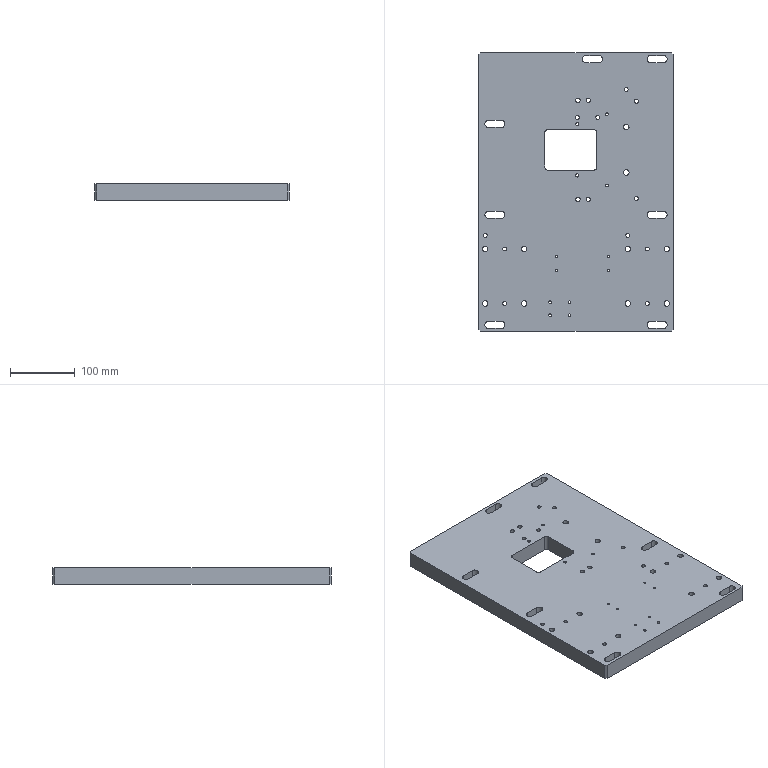CAM job | NX | 3-axis milling, drilling | part box 300 x 430 x 25 mm | stock box 300 x 430 x 25 mm
Tools:
number,name,description,diameter,corner_radius,flute_length,length,flutes
6,D6,平底铣刀-粗,6.0,0.0,25.0,75.0,2
9,D10,平底铣刀-粗,10.0,0.0,35.0,75.0,2
7,D6-J,平底铣刀-精,6.0,0.0,25.0,75.0,2
10,D10-J,平底铣刀-精,10.0,0.0,35.0,75.0,2
2,D6倒角刀,倒角刀,6.0,0.0,3.0,25.0,2
21,M4X0.7,丝锥,3.3,0.0,35.0,50.0,2
22,M5X0.8,丝锥,4.2,0.0,35.0,50.0,2
23,M6X1.0,丝锥,5.0,0.0,35.0,50.0,2
24,M8X1.25,丝锥,6.8,0.0,35.0,50.0,2
11,M10X1.5,丝锥,8.5,0.0,35.0,50.0,2
19,D6铰刀,Drilling Tool,6.0,0.0,75.0,100.0,6
1,C6定点钻,倒角刀,6.0,0.0,3.0,3.0,2
13,ZT3.4,钻头,3.4,0.0,35.0,50.0,2
15,ZT5.1,钻头,5.1,0.0,35.0,50.0,2
16,ZT6.8,钻头,6.8,0.0,35.0,50.0,2
17,ZT8.5,钻头,8.5,0.0,35.0,50.0,2
18,ZT5.9,Drilling Tool,5.9,0.0,35.0,50.0,2
20,ZT4.3,Drilling Tool,4.3,0.0,50.0,75.0,4
Operations:
program,operation,operation_type,tool,method,geometry_group,spindle_rpm,surface_speed,feed_per_tooth,feed_cut,feed_plunge,cut_length_mm,path_length_mm,cut_time_min,machine_time_min
B,CONSTANTZZIGZAGROUGH-MED_COPY_COPY,ZLevelMilling,D10,LAYEREDROUGH-DEPTHK-STEPOVERG,W-B,3000.0,94.245,0.3333,2000.0,100.0,3527.122,4789.797,1.764,1.89
B,DRILLCHAMFER_2,Operation,D6倒角刀,METHOD,W-B,2000.0,0.0,0.025,100.0,0.0,20.8,213.083,0.208,0.2272
B,DRILLCHAMFER_3,Operation,D6倒角刀,METHOD,W-B,2000.0,0.0,0.025,100.0,0.0,34.2,493.023,0.342,0.3879
B,MILLCHAMFER_6,PlanarMilling,D6倒角刀,METHOD,W-B,4000.0,75.398,0.0375,300.0,100.0,36.041,198.053,0.1201,0.1363
B,MILLCHAMFER_7,PlanarMilling,D6倒角刀,METHOD,W-B,4000.0,75.398,0.075,600.0,100.0,198.224,1451.821,0.3304,0.4557
B,MILLCHAMFER_8,PlanarMilling,D6倒角刀,METHOD,W-B,4000.0,75.398,0.0375,300.0,100.0,95.661,453.019,0.3189,0.3546
B,MILLCHAMFER_9,PlanarMilling,D6倒角刀,METHOD,W-B,3000.0,56.549,0.0667,400.0,100.0,351.512,1517.666,0.8788,0.9954
B,C0.3CLOSEDCONTOURCHAMFER6X45L_COPY,PlanarMilling,D6倒角刀,WALLCLIMB_CHAMFER-DEPTH0-STEPOVERG,W-B,4000.0,75.398,0.125,1000.0,100.0,2336.965,4238.784,2.337,2.527
B,CONSTANTZFINISH-MED_COPY_COPY,ZLevelMilling,D10-J,SIDEMILLFINISH-DEPTHK-STEPOVERG,W-B,3000.0,94.245,0.1333,800.0,100.0,44.032,1248.138,0.055,0.1755
A,CONSTANTZZIGZAGROUGH-MED_COPY,ZLevelMilling,D10,LAYEREDROUGH-DEPTHK-STEPOVERG,W-A,3000.0,94.245,0.3333,2000.0,100.0,3527.122,4885.722,1.764,1.899
A,SPOT-深0.8,Operation,C6定点钻,NONE,W-A,3000.0,56.0,0.01,60.0,90.0,91.8,2951.064,1.53,1.816
A,THROUGHHOLE-M4THREAD底孔,Operation,ZT3.4,NONE,W-A,1500.0,15.551,0.02,60.0,90.0,124.0,413.054,2.067,2.096
A,THROUGHHOLE-M5THREAD底孔,Operation,ZT4.3,NONE,W-A,1200.0,15.834,0.0333,80.0,90.0,186.0,786.035,2.325,2.385
A,THROUGHHOLE-M6THREAD底孔,Operation,ZT5.1,NONE,W-A,800.0,12.566,0.0625,100.0,90.0,64.0,248.006,0.64,0.6584
A,THROUGHHOLE-FINEHOLE6.0PREDRILL,Operation,ZT5.9,NONE,W-A,1000.0,18.535,0.04,80.0,90.0,337.735,1512.048,4.222,4.339
A,THROUGHHOLE-M8THREAD底孔,Operation,ZT6.8,NONE,W-A,600.0,12.818,0.1,120.0,90.0,134.172,496.409,1.118,1.154
A,THROUGHHOLE-M10THREAD底孔,Operation,ZT8.5,NONE,W-A,500.0,13.352,0.12,120.0,90.0,345.537,1496.159,2.88,2.994
A,POCKETROUGH_1,VolumeBased25DMillingOperation,D10,METHOD,W-A,3000.0,188.0,0.25,2500.0,80.0,25257.113,25320.413,10.103,10.109
A,THROUGHSLOTROUGH_1,VolumeBased25DMillingOperation,D6,METHOD,W-A,3500.0,113.0,0.2143,1500.0,100.0,39888.566,41342.031,26.592,26.738
A,SLOTFINISH_1,VolumeBased25DMillingOperation,D6-J,METHOD,W-A,3200.0,32.0,0.1143,600.0,100.0,2027.77,3991.606,3.38,3.576
A,DRILLCHAMFER_1,Operation,D6倒角刀,METHOD,W-A,4000.0,75.398,0.01,80.0,0.0,20.8,213.083,0.26,0.2792
A,MILLCHAMFER_1,PlanarMilling,D6倒角刀,METHOD,W-A,4000.0,75.398,0.025,200.0,100.0,108.122,725.825,0.5406,0.6024
A,MILLCHAMFER_2,PlanarMilling,D6倒角刀,METHOD,W-A,4000.0,75.398,0.0375,300.0,100.0,39.876,199.234,0.1329,0.1489
A,MILLCHAMFER_3,PlanarMilling,D6倒角刀,METHOD,W-A,4000.0,75.398,0.05,400.0,100.0,230.601,1473.006,0.5765,0.7007
A,MILLCHAMFER_4,PlanarMilling,D6倒角刀,METHOD,W-A,4000.0,75.398,0.0625,500.0,100.0,93.908,450.466,0.1878,0.2235
A,MILLCHAMFER_5,PlanarMilling,D6倒角刀,METHOD,W-A,4000.0,75.398,0.0625,500.0,100.0,344.337,1531.887,0.6887,0.8074
A,REAM,Operation,D6铰刀,METHOD,W-A,500.0,9.425,0.0167,50.0,0.0,297.0,1430.578,5.94,6.053
A,THROUGHHOLE-TAPM4,Operation,M4X0.7,METHOD,W-A,500.0,5.184,0.0007,0.7,90.0,118.0,401.054,168.571,168.6
A,THROUGHHOLE-TAPM5,Operation,M5X0.8,METHOD,W-A,500.0,6.597,0.0008,0.8,90.0,177.0,768.035,221.25,221.309
A,THROUGHHOLE-TAPM6,Operation,M6X1.0,METHOD,W-A,400.0,6.283,0.0013,1.0,90.0,59.0,238.006,59.0,59.018
A,THROUGHHOLE-TAPM8,Operation,M8X1.25,METHOD,W-A,300.0,6.409,0.0021,1.25,90.0,122.0,472.066,97.6,97.635
A,THROUGHHOLE-TAPM10,Operation,M10X1.5,METHOD,W-A,200.0,5.341,0.0037,1.5,90.0,310.0,1425.086,206.667,206.778
A,POCKETSEMIFINISH_1,VolumeBased25DMillingOperation,D6-J,METHOD,W-A,3200.0,157.0,0.2,800.0,90.0,793.823,882.687,0.9936,1.002
A,POCKETFINISH_1,VolumeBased25DMillingOperation,D6-J,METHOD,W-A,3200.0,157.0,0.2,800.0,90.0,263.722,352.322,0.33,0.3389
A,CONSTANTZFINISH-MED_COPY,ZLevelMilling,D10-J,SIDEMILLFINISH-DEPTHK-STEPOVERG,W-A,3000.0,94.245,0.1333,800.0,100.0,44.032,1217.299,0.055,0.1724